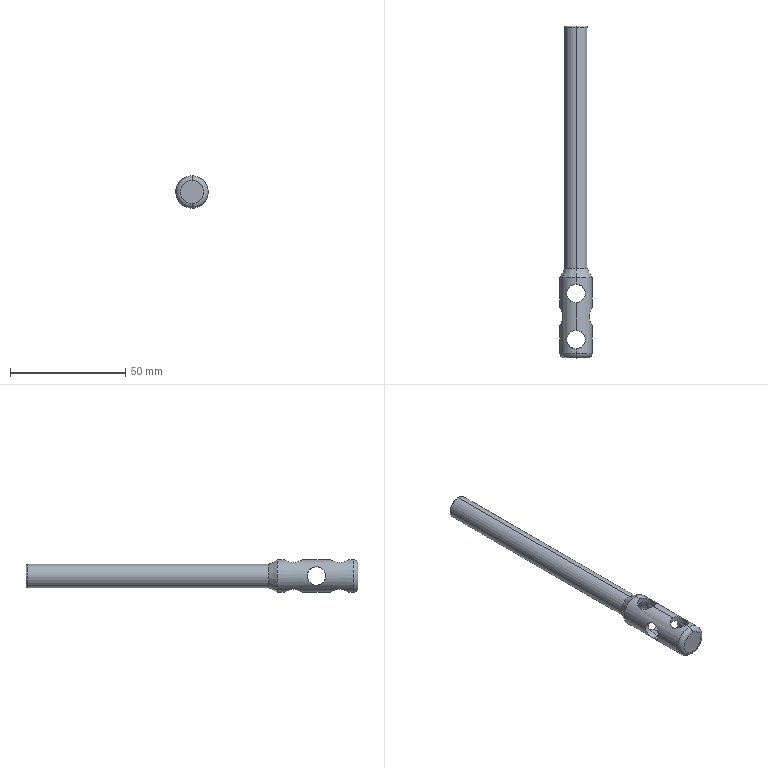Part | SolidWorks | features ICE 7, Fillet 2, Extrusion 1, MoveFace 1, Revolution 1 | 1 solid | 36 faces | box 14 x 144 x 14 mm | volume 6707 mm3 | cylinder 22 | torus 6 | cone 4 | plane 4 | commonest cylinder face diameters 8 x12 10 x4 6 x2 7 x2 14 x2